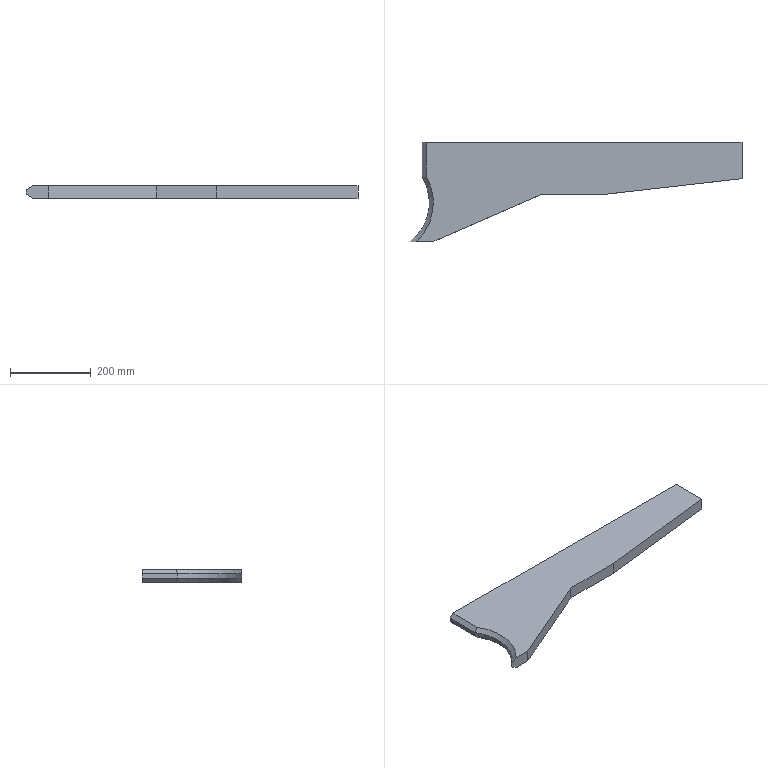Part | SolidWorks | features SplitBody 1 | 1 solid | 14 faces | box 823 x 246 x 30 mm | volume 3379824 mm3 | plane 11 | cone 2 | cylinder 1 | commonest cylinder face diameters 240 x1
STEP:
#1=CARTESIAN_POINT('',(3548.,918.44,1060.));
#2=VERTEX_POINT('',#1);
#3=CARTESIAN_POINT('',(3548.,834.44,1060.));
#4=VERTEX_POINT('',#3);
#5=CARTESIAN_POINT('',(3548.,768.44,1060.));
#6=DIRECTION('',(0.,-1.,0.));
#7=VECTOR('',#6,1000.);
#8=LINE('',#5,#7);
#9=EDGE_CURVE('',#2,#4,#8,.T.);
#10=ORIENTED_EDGE('',*,*,#9,.F.);
#11=CARTESIAN_POINT('',(4331.,918.44,1060.));
#12=VERTEX_POINT('',#11);
#13=CARTESIAN_POINT('',(3436.,918.44,1060.));
#14=DIRECTION('',(-1.,0.,0.));
#15=VECTOR('',#14,1000.);
#16=LINE('',#13,#15);
#17=EDGE_CURVE('',#12,#2,#16,.T.);
#18=ORIENTED_EDGE('',*,*,#17,.F.);
#19=CARTESIAN_POINT('',(4331.,828.44,1060.));
#20=VERTEX_POINT('',#19);
#21=CARTESIAN_POINT('',(4331.,768.44,1060.));
#22=DIRECTION('',(0.,1.,0.));
#23=VECTOR('',#22,1000.);
#24=LINE('',#21,#23);
#25=EDGE_CURVE('',#20,#12,#24,.T.);
#26=ORIENTED_EDGE('',*,*,#25,.F.);
#27=CARTESIAN_POINT('',(3981.,788.44,1060.));
#28=VERTEX_POINT('',#27);
#29=CARTESIAN_POINT('',(3981.,788.44,1060.));
#30=DIRECTION('',(0.9935,0.1135,0.));
#31=VECTOR('',#30,1000.);
#32=LINE('',#29,#31);
#33=EDGE_CURVE('',#28,#20,#32,.T.);
#34=ORIENTED_EDGE('',*,*,#33,.F.);
#35=CARTESIAN_POINT('',(3831.,788.44,1060.));
#36=VERTEX_POINT('',#35);
#37=CARTESIAN_POINT('',(3436.,788.44,1060.));
#38=DIRECTION('',(1.,0.,0.));
#39=VECTOR('',#38,1000.);
#40=LINE('',#37,#39);
#41=EDGE_CURVE('',#36,#28,#40,.T.);
#42=ORIENTED_EDGE('',*,*,#41,.F.);
#43=CARTESIAN_POINT('',(3565.,672.44,1060.));
#44=VERTEX_POINT('',#43);
#45=CARTESIAN_POINT('',(3565.,672.44,1060.));
#46=DIRECTION('',(0.9166,0.3997,0.));
#47=VECTOR('',#46,1000.);
#48=LINE('',#45,#47);
#49=EDGE_CURVE('',#44,#36,#48,.T.);
#50=ORIENTED_EDGE('',*,*,#49,.F.);
#51=CARTESIAN_POINT('',(3523.658,672.44,1060.));
#52=VERTEX_POINT('',#51);
#53=CARTESIAN_POINT('',(3436.,672.44,1060.));
#54=DIRECTION('',(1.,0.,0.));
#55=VECTOR('',#54,1000.);
#56=LINE('',#53,#55);
#57=EDGE_CURVE('',#52,#44,#56,.T.);
#58=ORIENTED_EDGE('',*,*,#57,.F.);
#59=CARTESIAN_POINT('',(3436.,768.44,1060.));
#60=DIRECTION('',(0.,0.,-1.));
#61=DIRECTION('',(-1.,0.,0.));
#62=AXIS2_PLACEMENT_3D('',#59,#60,#61);
#63=CIRCLE('',#62,130.);
#64=EDGE_CURVE('',#4,#52,#63,.T.);
#65=ORIENTED_EDGE('',*,*,#64,.F.);
#66=EDGE_LOOP('',(#10,#18,#26,#34,#42,#50,#58,#65));
#67=FACE_OUTER_BOUND('',#66,.T.);
#68=CARTESIAN_POINT('',(3436.,768.44,1060.));
#69=DIRECTION('',(0.,0.,1.));
#70=DIRECTION('',(1.,0.,0.));
#71=AXIS2_PLACEMENT_3D('',#68,#69,#70);
#72=PLANE('',#71);
#73=ADVANCED_FACE('',(#67),#72,.F.);
#74=CARTESIAN_POINT('',(3538.,831.654,1070.));
#75=VERTEX_POINT('',#74);
#76=CARTESIAN_POINT('',(3508.,672.44,1070.));
#77=VERTEX_POINT('',#76);
#78=CARTESIAN_POINT('',(3436.,768.44,1070.));
#79=DIRECTION('',(0.,0.,-1.));
#80=DIRECTION('',(-1.,0.,0.));
#81=AXIS2_PLACEMENT_3D('',#78,#79,#80);
#82=CIRCLE('',#81,120.);
#83=EDGE_CURVE('',#75,#77,#82,.T.);
#84=ORIENTED_EDGE('',*,*,#83,.F.);
#85=CARTESIAN_POINT('',(3548.,834.44,1060.));
#86=CARTESIAN_POINT('',(3544.595,833.511,1063.405));
#87=CARTESIAN_POINT('',(3541.261,832.583,1066.739));
#88=CARTESIAN_POINT('',(3538.,831.654,1070.));
#89=B_SPLINE_CURVE_WITH_KNOTS('',3,(#85,#86,#87,#88),.UNSPECIFIED.,.F.,.F.,(4,4),(0.,1.),.UNSPECIFIED.);
#90=EDGE_CURVE('',#4,#75,#89,.T.);
#91=ORIENTED_EDGE('',*,*,#90,.F.);
#92=ORIENTED_EDGE('',*,*,#64,.T.);
#93=CARTESIAN_POINT('',(3508.,672.44,1070.));
#94=CARTESIAN_POINT('',(3513.313,672.44,1066.812));
#95=CARTESIAN_POINT('',(3518.522,672.44,1063.463));
#96=CARTESIAN_POINT('',(3523.658,672.44,1060.));
#97=B_SPLINE_CURVE_WITH_KNOTS('',3,(#93,#94,#95,#96),.UNSPECIFIED.,.F.,.F.,(4,4),(0.,0.01858),.UNSPECIFIED.);
#98=EDGE_CURVE('',#77,#52,#97,.T.);
#99=ORIENTED_EDGE('',*,*,#98,.F.);
#100=EDGE_LOOP('',(#84,#91,#92,#99));
#101=FACE_OUTER_BOUND('',#100,.T.);
#102=CARTESIAN_POINT('',(3436.,768.44,1060.));
#103=DIRECTION('',(0.,0.,-1.));
#104=DIRECTION('',(-1.,0.,0.));
#105=AXIS2_PLACEMENT_3D('',#102,#103,#104);
#106=CONICAL_SURFACE('',#105,130.,0.7854);
#107=ADVANCED_FACE('',(#101),#106,.F.);
#108=ORIENTED_EDGE('',*,*,#9,.T.);
#109=ORIENTED_EDGE('',*,*,#90,.T.);
#110=CARTESIAN_POINT('',(3538.,918.44,1070.));
#111=VERTEX_POINT('',#110);
#112=CARTESIAN_POINT('',(3538.,918.44,1070.));
#113=DIRECTION('',(0.,-1.,0.));
#114=VECTOR('',#113,1000.);
#115=LINE('',#112,#114);
#116=EDGE_CURVE('',#111,#75,#115,.T.);
#117=ORIENTED_EDGE('',*,*,#116,.F.);
#118=CARTESIAN_POINT('',(3538.,918.44,1070.));
#119=DIRECTION('',(-0.7071,0.,0.7071));
#120=VECTOR('',#119,1000.);
#121=LINE('',#118,#120);
#122=EDGE_CURVE('',#2,#111,#121,.T.);
#123=ORIENTED_EDGE('',*,*,#122,.F.);
#124=EDGE_LOOP('',(#108,#109,#117,#123));
#125=FACE_OUTER_BOUND('',#124,.T.);
#126=CARTESIAN_POINT('',(3538.,918.44,1070.));
#127=DIRECTION('',(0.7071,0.,0.7071));
#128=DIRECTION('',(0.7071,0.,-0.7071));
#129=AXIS2_PLACEMENT_3D('',#126,#127,#128);
#130=PLANE('',#129);
#131=ADVANCED_FACE('',(#125),#130,.F.);
#132=ORIENTED_EDGE('',*,*,#122,.T.);
#133=CARTESIAN_POINT('',(3538.,918.44,1080.));
#134=VERTEX_POINT('',#133);
#135=CARTESIAN_POINT('',(3538.,918.44,1090.));
#136=DIRECTION('',(0.,0.,-1.));
#137=VECTOR('',#136,1000.);
#138=LINE('',#135,#137);
#139=EDGE_CURVE('',#134,#111,#138,.T.);
#140=ORIENTED_EDGE('',*,*,#139,.F.);
#141=CARTESIAN_POINT('',(3548.,918.44,1090.));
#142=VERTEX_POINT('',#141);
#143=CARTESIAN_POINT('',(3548.,918.44,1090.));
#144=DIRECTION('',(-0.7071,0.,-0.7071));
#145=VECTOR('',#144,1000.);
#146=LINE('',#143,#145);
#147=EDGE_CURVE('',#142,#134,#146,.T.);
#148=ORIENTED_EDGE('',*,*,#147,.F.);
#149=CARTESIAN_POINT('',(4331.,918.44,1090.));
#150=VERTEX_POINT('',#149);
#151=CARTESIAN_POINT('',(3538.,918.44,1090.));
#152=DIRECTION('',(-1.,0.,0.));
#153=VECTOR('',#152,1000.);
#154=LINE('',#151,#153);
#155=EDGE_CURVE('',#150,#142,#154,.T.);
#156=ORIENTED_EDGE('',*,*,#155,.F.);
#157=CARTESIAN_POINT('',(4331.,918.44,1090.));
#158=DIRECTION('',(0.,0.,1.));
#159=VECTOR('',#158,1000.);
#160=LINE('',#157,#159);
#161=EDGE_CURVE('',#12,#150,#160,.T.);
#162=ORIENTED_EDGE('',*,*,#161,.F.);
#163=ORIENTED_EDGE('',*,*,#17,.T.);
#164=EDGE_LOOP('',(#132,#140,#148,#156,#162,#163));
#165=FACE_OUTER_BOUND('',#164,.T.);
#166=CARTESIAN_POINT('',(3538.,918.44,1090.));
#167=DIRECTION('',(0.,-1.,0.));
#168=DIRECTION('',(0.,0.,-1.));
#169=AXIS2_PLACEMENT_3D('',#166,#167,#168);
#170=PLANE('',#169);
#171=ADVANCED_FACE('',(#165),#170,.F.);
#172=ORIENTED_EDGE('',*,*,#161,.T.);
#173=CARTESIAN_POINT('',(4331.,828.44,1090.));
#174=VERTEX_POINT('',#173);
#175=CARTESIAN_POINT('',(4331.,918.44,1090.));
#176=DIRECTION('',(0.,1.,0.));
#177=VECTOR('',#176,1000.);
#178=LINE('',#175,#177);
#179=EDGE_CURVE('',#174,#150,#178,.T.);
#180=ORIENTED_EDGE('',*,*,#179,.F.);
#181=CARTESIAN_POINT('',(4331.,828.44,1090.));
#182=DIRECTION('',(0.,0.,1.));
#183=VECTOR('',#182,1000.);
#184=LINE('',#181,#183);
#185=EDGE_CURVE('',#20,#174,#184,.T.);
#186=ORIENTED_EDGE('',*,*,#185,.F.);
#187=ORIENTED_EDGE('',*,*,#25,.T.);
#188=EDGE_LOOP('',(#172,#180,#186,#187));
#189=FACE_OUTER_BOUND('',#188,.T.);
#190=CARTESIAN_POINT('',(4331.,918.44,1090.));
#191=DIRECTION('',(-1.,0.,0.));
#192=DIRECTION('',(0.,0.,1.));
#193=AXIS2_PLACEMENT_3D('',#190,#191,#192);
#194=PLANE('',#193);
#195=ADVANCED_FACE('',(#189),#194,.F.);
#196=ORIENTED_EDGE('',*,*,#185,.T.);
#197=CARTESIAN_POINT('',(3981.,788.44,1090.));
#198=VERTEX_POINT('',#197);
#199=CARTESIAN_POINT('',(4331.,828.44,1090.));
#200=DIRECTION('',(0.9935,0.1135,0.));
#201=VECTOR('',#200,1000.);
#202=LINE('',#199,#201);
#203=EDGE_CURVE('',#198,#174,#202,.T.);
#204=ORIENTED_EDGE('',*,*,#203,.F.);
#205=CARTESIAN_POINT('',(3981.,788.44,1090.));
#206=DIRECTION('',(0.,0.,1.));
#207=VECTOR('',#206,1000.);
#208=LINE('',#205,#207);
#209=EDGE_CURVE('',#28,#198,#208,.T.);
#210=ORIENTED_EDGE('',*,*,#209,.F.);
#211=ORIENTED_EDGE('',*,*,#33,.T.);
#212=EDGE_LOOP('',(#196,#204,#210,#211));
#213=FACE_OUTER_BOUND('',#212,.T.);
#214=CARTESIAN_POINT('',(4331.,828.44,1090.));
#215=DIRECTION('',(-0.1135,0.9935,0.));
#216=DIRECTION('',(-0.9935,-0.1135,0.));
#217=AXIS2_PLACEMENT_3D('',#214,#215,#216);
#218=PLANE('',#217);
#219=ADVANCED_FACE('',(#213),#218,.F.);
#220=ORIENTED_EDGE('',*,*,#209,.T.);
#221=CARTESIAN_POINT('',(3831.,788.44,1090.));
#222=VERTEX_POINT('',#221);
#223=CARTESIAN_POINT('',(3981.,788.44,1090.));
#224=DIRECTION('',(1.,0.,0.));
#225=VECTOR('',#224,1000.);
#226=LINE('',#223,#225);
#227=EDGE_CURVE('',#222,#198,#226,.T.);
#228=ORIENTED_EDGE('',*,*,#227,.F.);
#229=CARTESIAN_POINT('',(3831.,788.44,1090.));
#230=DIRECTION('',(0.,0.,1.));
#231=VECTOR('',#230,1000.);
#232=LINE('',#229,#231);
#233=EDGE_CURVE('',#36,#222,#232,.T.);
#234=ORIENTED_EDGE('',*,*,#233,.F.);
#235=ORIENTED_EDGE('',*,*,#41,.T.);
#236=EDGE_LOOP('',(#220,#228,#234,#235));
#237=FACE_OUTER_BOUND('',#236,.T.);
#238=CARTESIAN_POINT('',(3981.,788.44,1090.));
#239=DIRECTION('',(0.,1.,0.));
#240=DIRECTION('',(-1.,0.,0.));
#241=AXIS2_PLACEMENT_3D('',#238,#239,#240);
#242=PLANE('',#241);
#243=ADVANCED_FACE('',(#237),#242,.F.);
#244=ORIENTED_EDGE('',*,*,#233,.T.);
#245=CARTESIAN_POINT('',(3565.,672.44,1090.));
#246=VERTEX_POINT('',#245);
#247=CARTESIAN_POINT('',(3565.,672.44,1090.));
#248=DIRECTION('',(0.9166,0.3997,0.));
#249=VECTOR('',#248,1000.);
#250=LINE('',#247,#249);
#251=EDGE_CURVE('',#246,#222,#250,.T.);
#252=ORIENTED_EDGE('',*,*,#251,.F.);
#253=CARTESIAN_POINT('',(3565.,672.44,1090.));
#254=DIRECTION('',(0.,0.,1.));
#255=VECTOR('',#254,1000.);
#256=LINE('',#253,#255);
#257=EDGE_CURVE('',#44,#246,#256,.T.);
#258=ORIENTED_EDGE('',*,*,#257,.F.);
#259=ORIENTED_EDGE('',*,*,#49,.T.);
#260=EDGE_LOOP('',(#244,#252,#258,#259));
#261=FACE_OUTER_BOUND('',#260,.T.);
#262=CARTESIAN_POINT('',(3565.,672.44,1090.));
#263=DIRECTION('',(-0.3997,0.9166,0.));
#264=DIRECTION('',(-0.9166,-0.3997,0.));
#265=AXIS2_PLACEMENT_3D('',#262,#263,#264);
#266=PLANE('',#265);
#267=ADVANCED_FACE('',(#261),#266,.F.);
#268=ORIENTED_EDGE('',*,*,#98,.T.);
#269=ORIENTED_EDGE('',*,*,#57,.T.);
#270=ORIENTED_EDGE('',*,*,#257,.T.);
#271=CARTESIAN_POINT('',(3523.658,672.44,1090.));
#272=VERTEX_POINT('',#271);
#273=CARTESIAN_POINT('',(3565.,672.44,1090.));
#274=DIRECTION('',(1.,0.,0.));
#275=VECTOR('',#274,1000.);
#276=LINE('',#273,#275);
#277=EDGE_CURVE('',#272,#246,#276,.T.);
#278=ORIENTED_EDGE('',*,*,#277,.F.);
#279=CARTESIAN_POINT('',(3508.,672.44,1080.));
#280=VERTEX_POINT('',#279);
#281=CARTESIAN_POINT('',(3508.,672.44,1080.));
#282=CARTESIAN_POINT('',(3513.313,672.44,1083.188));
#283=CARTESIAN_POINT('',(3518.522,672.44,1086.537));
#284=CARTESIAN_POINT('',(3523.658,672.44,1090.));
#285=B_SPLINE_CURVE_WITH_KNOTS('',3,(#281,#282,#283,#284),.UNSPECIFIED.,.F.,.F.,(4,4),(0.,0.01858),.UNSPECIFIED.);
#286=EDGE_CURVE('',#280,#272,#285,.T.);
#287=ORIENTED_EDGE('',*,*,#286,.F.);
#288=CARTESIAN_POINT('',(3508.,672.44,1090.));
#289=DIRECTION('',(0.,0.,1.));
#290=VECTOR('',#289,1000.);
#291=LINE('',#288,#290);
#292=EDGE_CURVE('',#77,#280,#291,.T.);
#293=ORIENTED_EDGE('',*,*,#292,.F.);
#294=EDGE_LOOP('',(#268,#269,#270,#278,#287,#293));
#295=FACE_OUTER_BOUND('',#294,.T.);
#296=CARTESIAN_POINT('',(3565.,672.44,1090.));
#297=DIRECTION('',(0.,1.,0.));
#298=DIRECTION('',(-1.,0.,0.));
#299=AXIS2_PLACEMENT_3D('',#296,#297,#298);
#300=PLANE('',#299);
#301=ADVANCED_FACE('',(#295),#300,.F.);
#302=ORIENTED_EDGE('',*,*,#83,.T.);
#303=ORIENTED_EDGE('',*,*,#292,.T.);
#304=CARTESIAN_POINT('',(3538.,831.654,1080.));
#305=VERTEX_POINT('',#304);
#306=CARTESIAN_POINT('',(3436.,768.44,1080.));
#307=DIRECTION('',(0.,0.,-1.));
#308=DIRECTION('',(-1.,0.,0.));
#309=AXIS2_PLACEMENT_3D('',#306,#307,#308);
#310=CIRCLE('',#309,120.);
#311=EDGE_CURVE('',#305,#280,#310,.T.);
#312=ORIENTED_EDGE('',*,*,#311,.F.);
#313=CARTESIAN_POINT('',(3538.,831.654,1090.));
#314=DIRECTION('',(0.,0.,1.));
#315=VECTOR('',#314,1000.);
#316=LINE('',#313,#315);
#317=EDGE_CURVE('',#75,#305,#316,.T.);
#318=ORIENTED_EDGE('',*,*,#317,.F.);
#319=EDGE_LOOP('',(#302,#303,#312,#318));
#320=FACE_OUTER_BOUND('',#319,.T.);
#321=CARTESIAN_POINT('',(3436.,768.44,1090.));
#322=DIRECTION('',(0.,0.,-1.));
#323=DIRECTION('',(-1.,0.,0.));
#324=AXIS2_PLACEMENT_3D('',#321,#322,#323);
#325=CYLINDRICAL_SURFACE('',#324,120.);
#326=ADVANCED_FACE('',(#320),#325,.F.);
#327=ORIENTED_EDGE('',*,*,#116,.T.);
#328=ORIENTED_EDGE('',*,*,#317,.T.);
#329=CARTESIAN_POINT('',(3538.,918.44,1080.));
#330=DIRECTION('',(0.,-1.,0.));
#331=VECTOR('',#330,1000.);
#332=LINE('',#329,#331);
#333=EDGE_CURVE('',#134,#305,#332,.T.);
#334=ORIENTED_EDGE('',*,*,#333,.F.);
#335=ORIENTED_EDGE('',*,*,#139,.T.);
#336=EDGE_LOOP('',(#327,#328,#334,#335));
#337=FACE_OUTER_BOUND('',#336,.T.);
#338=CARTESIAN_POINT('',(3538.,918.44,1090.));
#339=DIRECTION('',(1.,0.,0.));
#340=DIRECTION('',(0.,0.,-1.));
#341=AXIS2_PLACEMENT_3D('',#338,#339,#340);
#342=PLANE('',#341);
#343=ADVANCED_FACE('',(#337),#342,.F.);
#344=CARTESIAN_POINT('',(3548.,834.44,1090.));
#345=VERTEX_POINT('',#344);
#346=CARTESIAN_POINT('',(3538.,831.654,1080.));
#347=CARTESIAN_POINT('',(3541.261,832.583,1083.261));
#348=CARTESIAN_POINT('',(3544.595,833.511,1086.595));
#349=CARTESIAN_POINT('',(3548.,834.44,1090.));
#350=B_SPLINE_CURVE_WITH_KNOTS('',3,(#346,#347,#348,#349),.UNSPECIFIED.,.F.,.F.,(4,4),(0.,1.),.UNSPECIFIED.);
#351=EDGE_CURVE('',#305,#345,#350,.T.);
#352=ORIENTED_EDGE('',*,*,#351,.T.);
#353=CARTESIAN_POINT('',(3548.,768.44,1090.));
#354=DIRECTION('',(0.,1.,0.));
#355=VECTOR('',#354,1000.);
#356=LINE('',#353,#355);
#357=EDGE_CURVE('',#345,#142,#356,.T.);
#358=ORIENTED_EDGE('',*,*,#357,.T.);
#359=ORIENTED_EDGE('',*,*,#147,.T.);
#360=ORIENTED_EDGE('',*,*,#333,.T.);
#361=EDGE_LOOP('',(#352,#358,#359,#360));
#362=FACE_OUTER_BOUND('',#361,.T.);
#363=CARTESIAN_POINT('',(3548.,768.44,1090.));
#364=DIRECTION('',(-0.7071,0.,0.7071));
#365=DIRECTION('',(0.7071,0.,0.7071));
#366=AXIS2_PLACEMENT_3D('',#363,#364,#365);
#367=PLANE('',#366);
#368=ADVANCED_FACE('',(#362),#367,.T.);
#369=ORIENTED_EDGE('',*,*,#179,.T.);
#370=ORIENTED_EDGE('',*,*,#155,.T.);
#371=ORIENTED_EDGE('',*,*,#357,.F.);
#372=CARTESIAN_POINT('',(3436.,768.44,1090.));
#373=DIRECTION('',(0.,0.,-1.));
#374=DIRECTION('',(0.,-1.,0.));
#375=AXIS2_PLACEMENT_3D('',#372,#373,#374);
#376=CIRCLE('',#375,130.);
#377=EDGE_CURVE('',#345,#272,#376,.T.);
#378=ORIENTED_EDGE('',*,*,#377,.T.);
#379=ORIENTED_EDGE('',*,*,#277,.T.);
#380=ORIENTED_EDGE('',*,*,#251,.T.);
#381=ORIENTED_EDGE('',*,*,#227,.T.);
#382=ORIENTED_EDGE('',*,*,#203,.T.);
#383=EDGE_LOOP('',(#369,#370,#371,#378,#379,#380,#381,#382));
#384=FACE_OUTER_BOUND('',#383,.T.);
#385=CARTESIAN_POINT('',(3436.,768.44,1090.));
#386=DIRECTION('',(0.,0.,1.));
#387=DIRECTION('',(1.,0.,0.));
#388=AXIS2_PLACEMENT_3D('',#385,#386,#387);
#389=PLANE('',#388);
#390=ADVANCED_FACE('',(#384),#389,.T.);
#391=ORIENTED_EDGE('',*,*,#311,.T.);
#392=ORIENTED_EDGE('',*,*,#286,.T.);
#393=ORIENTED_EDGE('',*,*,#377,.F.);
#394=ORIENTED_EDGE('',*,*,#351,.F.);
#395=EDGE_LOOP('',(#391,#392,#393,#394));
#396=FACE_OUTER_BOUND('',#395,.T.);
#397=CARTESIAN_POINT('',(3436.,768.44,1090.));
#398=DIRECTION('',(0.,0.,1.));
#399=DIRECTION('',(0.,-1.,0.));
#400=AXIS2_PLACEMENT_3D('',#397,#398,#399);
#401=CONICAL_SURFACE('',#400,130.,0.7854);
#402=ADVANCED_FACE('',(#396),#401,.F.);
#403=CLOSED_SHELL('',(#73,#107,#131,#171,#195,#219,#243,#267,#301,#326,#343,#368,#390,#402));
#404=MANIFOLD_SOLID_BREP('',#403);
#405=CARTESIAN_POINT('',(0.,0.,0.));
#406=DIRECTION('',(0.,0.,1.));
#407=DIRECTION('',(1.,0.,0.));
#408=AXIS2_PLACEMENT_3D('',#405,#406,#407);
#409=(LENGTH_UNIT()NAMED_UNIT(*)SI_UNIT(.MILLI.,.METRE.));
#410=UNCERTAINTY_MEASURE_WITH_UNIT(LENGTH_MEASURE(0.00001),#409,'','');
#411=(NAMED_UNIT(*)PLANE_ANGLE_UNIT()SI_UNIT($,.RADIAN.));
#412=(NAMED_UNIT(*)SI_UNIT($,.STERADIAN.)SOLID_ANGLE_UNIT());
#413=(GEOMETRIC_REPRESENTATION_CONTEXT(3)GLOBAL_UNCERTAINTY_ASSIGNED_CONTEXT((#410))GLOBAL_UNIT_ASSIGNED_CONTEXT((#409,#411,#412))REPRESENTATION_CONTEXT('',''));
#414=ADVANCED_BREP_SHAPE_REPRESENTATION('',(#404,#408),#413);